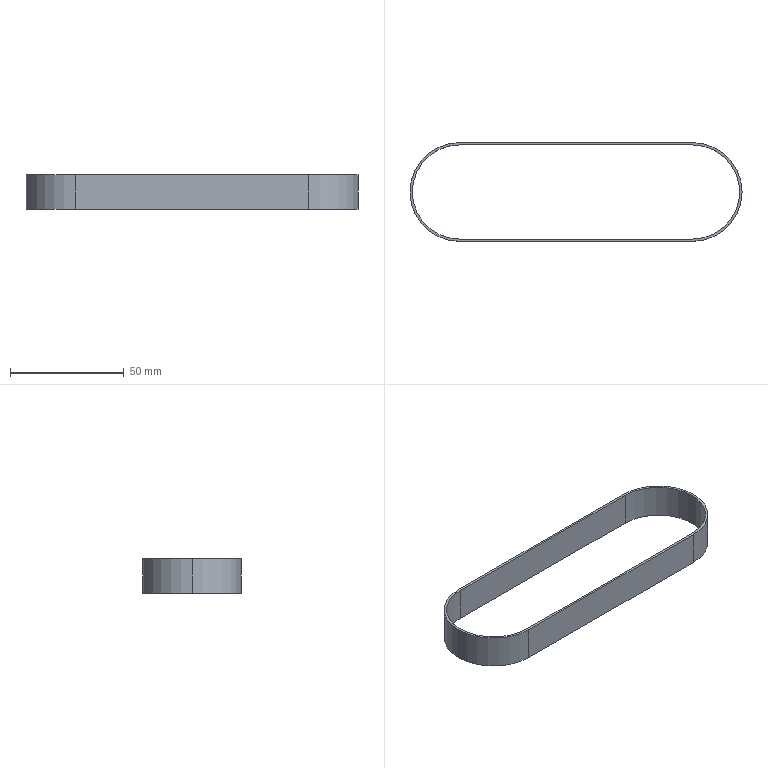Part | STEP file | Timing belt TTBU325T5-150_MISUMI | 1 solid | 12 faces | box 145.88 x 43.38 x 15 mm | volume 5072 mm3 | cylinder 6 | plane 6 | commonest cylinder face diameters 41.38 x3 43.38 x3
STEP:
#1=CARTESIAN_POINT('',(-21.69,0.,15.));
#2=VERTEX_POINT('',#1);
#3=CARTESIAN_POINT('',(0.,-21.69,15.));
#4=VERTEX_POINT('',#3);
#5=CARTESIAN_POINT('',(0.,0.,15.));
#6=DIRECTION('',(0.,0.,1.));
#7=DIRECTION('',(-1.,0.,0.));
#8=AXIS2_PLACEMENT_3D('',#5,#6,#7);
#9=CIRCLE('',#8,21.69);
#10=EDGE_CURVE('',#2,#4,#9,.T.);
#11=ORIENTED_EDGE('',*,*,#10,.F.);
#12=CARTESIAN_POINT('',(-21.69,0.,0.));
#13=VERTEX_POINT('',#12);
#14=CARTESIAN_POINT('',(-21.69,0.,15.));
#15=DIRECTION('',(0.,0.,-1.));
#16=VECTOR('',#15,1000.);
#17=LINE('',#14,#16);
#18=EDGE_CURVE('',#2,#13,#17,.T.);
#19=ORIENTED_EDGE('',*,*,#18,.T.);
#20=CARTESIAN_POINT('',(0.,-21.69,0.));
#21=VERTEX_POINT('',#20);
#22=CARTESIAN_POINT('',(0.,0.,0.));
#23=DIRECTION('',(0.,0.,1.));
#24=DIRECTION('',(-1.,0.,0.));
#25=AXIS2_PLACEMENT_3D('',#22,#23,#24);
#26=CIRCLE('',#25,21.69);
#27=EDGE_CURVE('',#13,#21,#26,.T.);
#28=ORIENTED_EDGE('',*,*,#27,.T.);
#29=CARTESIAN_POINT('',(0.,-21.69,15.));
#30=DIRECTION('',(0.,0.,1.));
#31=VECTOR('',#30,1000.);
#32=LINE('',#29,#31);
#33=EDGE_CURVE('',#21,#4,#32,.T.);
#34=ORIENTED_EDGE('',*,*,#33,.T.);
#35=EDGE_LOOP('',(#11,#19,#28,#34));
#36=FACE_OUTER_BOUND('',#35,.T.);
#37=CARTESIAN_POINT('',(0.,0.,15.));
#38=DIRECTION('',(0.,0.,-1.));
#39=DIRECTION('',(-1.,0.,0.));
#40=AXIS2_PLACEMENT_3D('',#37,#38,#39);
#41=CYLINDRICAL_SURFACE('',#40,21.69);
#42=ADVANCED_FACE('',(#36),#41,.T.);
#43=CARTESIAN_POINT('',(-20.69,0.,15.));
#44=VERTEX_POINT('',#43);
#45=CARTESIAN_POINT('',(0.,20.69,15.));
#46=VERTEX_POINT('',#45);
#47=CARTESIAN_POINT('',(0.,0.,15.));
#48=DIRECTION('',(0.,0.,-1.));
#49=DIRECTION('',(-1.,0.,0.));
#50=AXIS2_PLACEMENT_3D('',#47,#48,#49);
#51=CIRCLE('',#50,20.69);
#52=EDGE_CURVE('',#44,#46,#51,.T.);
#53=ORIENTED_EDGE('',*,*,#52,.F.);
#54=CARTESIAN_POINT('',(-20.69,0.,0.));
#55=VERTEX_POINT('',#54);
#56=CARTESIAN_POINT('',(-20.69,0.,15.));
#57=DIRECTION('',(0.,0.,-1.));
#58=VECTOR('',#57,1000.);
#59=LINE('',#56,#58);
#60=EDGE_CURVE('',#44,#55,#59,.T.);
#61=ORIENTED_EDGE('',*,*,#60,.T.);
#62=CARTESIAN_POINT('',(0.,20.69,0.));
#63=VERTEX_POINT('',#62);
#64=CARTESIAN_POINT('',(0.,0.,0.));
#65=DIRECTION('',(0.,0.,-1.));
#66=DIRECTION('',(-1.,0.,0.));
#67=AXIS2_PLACEMENT_3D('',#64,#65,#66);
#68=CIRCLE('',#67,20.69);
#69=EDGE_CURVE('',#55,#63,#68,.T.);
#70=ORIENTED_EDGE('',*,*,#69,.T.);
#71=CARTESIAN_POINT('',(0.,20.69,15.));
#72=DIRECTION('',(0.,0.,-1.));
#73=VECTOR('',#72,1000.);
#74=LINE('',#71,#73);
#75=EDGE_CURVE('',#46,#63,#74,.T.);
#76=ORIENTED_EDGE('',*,*,#75,.F.);
#77=EDGE_LOOP('',(#53,#61,#70,#76));
#78=FACE_OUTER_BOUND('',#77,.T.);
#79=CARTESIAN_POINT('',(0.,0.,15.));
#80=DIRECTION('',(0.,0.,-1.));
#81=DIRECTION('',(-1.,0.,0.));
#82=AXIS2_PLACEMENT_3D('',#79,#80,#81);
#83=CYLINDRICAL_SURFACE('',#82,20.69);
#84=ADVANCED_FACE('',(#78),#83,.F.);
#85=CARTESIAN_POINT('',(102.5,-21.69,15.));
#86=VERTEX_POINT('',#85);
#87=CARTESIAN_POINT('',(102.5,-21.69,0.));
#88=VERTEX_POINT('',#87);
#89=CARTESIAN_POINT('',(102.5,-21.69,15.));
#90=DIRECTION('',(0.,0.,-1.));
#91=VECTOR('',#90,1000.);
#92=LINE('',#89,#91);
#93=EDGE_CURVE('',#86,#88,#92,.T.);
#94=ORIENTED_EDGE('',*,*,#93,.F.);
#95=CARTESIAN_POINT('',(0.,-21.69,15.));
#96=DIRECTION('',(1.,0.,0.));
#97=VECTOR('',#96,1000.);
#98=LINE('',#95,#97);
#99=EDGE_CURVE('',#4,#86,#98,.T.);
#100=ORIENTED_EDGE('',*,*,#99,.F.);
#101=ORIENTED_EDGE('',*,*,#33,.F.);
#102=CARTESIAN_POINT('',(0.,-21.69,0.));
#103=DIRECTION('',(-1.,0.,0.));
#104=VECTOR('',#103,1000.);
#105=LINE('',#102,#104);
#106=EDGE_CURVE('',#88,#21,#105,.T.);
#107=ORIENTED_EDGE('',*,*,#106,.F.);
#108=EDGE_LOOP('',(#94,#100,#101,#107));
#109=FACE_OUTER_BOUND('',#108,.T.);
#110=CARTESIAN_POINT('',(0.,-21.69,15.));
#111=DIRECTION('',(0.,1.,0.));
#112=DIRECTION('',(0.,0.,1.));
#113=AXIS2_PLACEMENT_3D('',#110,#111,#112);
#114=PLANE('',#113);
#115=ADVANCED_FACE('',(#109),#114,.F.);
#116=CARTESIAN_POINT('',(0.,-20.69,0.));
#117=VERTEX_POINT('',#116);
#118=CARTESIAN_POINT('',(0.,0.,0.));
#119=DIRECTION('',(0.,0.,-1.));
#120=DIRECTION('',(-1.,0.,0.));
#121=AXIS2_PLACEMENT_3D('',#118,#119,#120);
#122=CIRCLE('',#121,20.69);
#123=EDGE_CURVE('',#117,#55,#122,.T.);
#124=ORIENTED_EDGE('',*,*,#123,.F.);
#125=CARTESIAN_POINT('',(102.5,-20.69,0.));
#126=VERTEX_POINT('',#125);
#127=CARTESIAN_POINT('',(0.,-20.69,0.));
#128=DIRECTION('',(-1.,0.,0.));
#129=VECTOR('',#128,1000.);
#130=LINE('',#127,#129);
#131=EDGE_CURVE('',#126,#117,#130,.T.);
#132=ORIENTED_EDGE('',*,*,#131,.F.);
#133=CARTESIAN_POINT('',(102.5,20.69,0.));
#134=VERTEX_POINT('',#133);
#135=CARTESIAN_POINT('',(102.5,0.,0.));
#136=DIRECTION('',(0.,0.,-1.));
#137=DIRECTION('',(-1.,0.,0.));
#138=AXIS2_PLACEMENT_3D('',#135,#136,#137);
#139=CIRCLE('',#138,20.69);
#140=EDGE_CURVE('',#134,#126,#139,.T.);
#141=ORIENTED_EDGE('',*,*,#140,.F.);
#142=CARTESIAN_POINT('',(0.,20.69,0.));
#143=DIRECTION('',(1.,0.,0.));
#144=VECTOR('',#143,1000.);
#145=LINE('',#142,#144);
#146=EDGE_CURVE('',#63,#134,#145,.T.);
#147=ORIENTED_EDGE('',*,*,#146,.F.);
#148=ORIENTED_EDGE('',*,*,#69,.F.);
#149=EDGE_LOOP('',(#124,#132,#141,#147,#148));
#150=FACE_BOUND('',#149,.T.);
#151=CARTESIAN_POINT('',(102.5,21.69,0.));
#152=VERTEX_POINT('',#151);
#153=CARTESIAN_POINT('',(0.,21.69,0.));
#154=VERTEX_POINT('',#153);
#155=CARTESIAN_POINT('',(0.,21.69,0.));
#156=DIRECTION('',(-1.,0.,0.));
#157=VECTOR('',#156,1000.);
#158=LINE('',#155,#157);
#159=EDGE_CURVE('',#152,#154,#158,.T.);
#160=ORIENTED_EDGE('',*,*,#159,.F.);
#161=CARTESIAN_POINT('',(102.5,0.,0.));
#162=DIRECTION('',(0.,0.,1.));
#163=DIRECTION('',(-1.,0.,0.));
#164=AXIS2_PLACEMENT_3D('',#161,#162,#163);
#165=CIRCLE('',#164,21.69);
#166=EDGE_CURVE('',#88,#152,#165,.T.);
#167=ORIENTED_EDGE('',*,*,#166,.F.);
#168=ORIENTED_EDGE('',*,*,#106,.T.);
#169=ORIENTED_EDGE('',*,*,#27,.F.);
#170=CARTESIAN_POINT('',(0.,0.,0.));
#171=DIRECTION('',(0.,0.,1.));
#172=DIRECTION('',(-1.,0.,0.));
#173=AXIS2_PLACEMENT_3D('',#170,#171,#172);
#174=CIRCLE('',#173,21.69);
#175=EDGE_CURVE('',#154,#13,#174,.T.);
#176=ORIENTED_EDGE('',*,*,#175,.F.);
#177=EDGE_LOOP('',(#160,#167,#168,#169,#176));
#178=FACE_OUTER_BOUND('',#177,.T.);
#179=CARTESIAN_POINT('',(0.,0.,0.));
#180=DIRECTION('',(0.,0.,1.));
#181=DIRECTION('',(1.,0.,0.));
#182=AXIS2_PLACEMENT_3D('',#179,#180,#181);
#183=PLANE('',#182);
#184=ADVANCED_FACE('',(#150,#178),#183,.F.);
#185=CARTESIAN_POINT('',(102.5,21.69,15.));
#186=VERTEX_POINT('',#185);
#187=CARTESIAN_POINT('',(102.5,0.,15.));
#188=DIRECTION('',(0.,0.,-1.));
#189=DIRECTION('',(-1.,0.,0.));
#190=AXIS2_PLACEMENT_3D('',#187,#188,#189);
#191=CIRCLE('',#190,21.69);
#192=EDGE_CURVE('',#186,#86,#191,.T.);
#193=ORIENTED_EDGE('',*,*,#192,.T.);
#194=ORIENTED_EDGE('',*,*,#93,.T.);
#195=ORIENTED_EDGE('',*,*,#166,.T.);
#196=CARTESIAN_POINT('',(102.5,21.69,15.));
#197=DIRECTION('',(0.,0.,1.));
#198=VECTOR('',#197,1000.);
#199=LINE('',#196,#198);
#200=EDGE_CURVE('',#152,#186,#199,.T.);
#201=ORIENTED_EDGE('',*,*,#200,.T.);
#202=EDGE_LOOP('',(#193,#194,#195,#201));
#203=FACE_OUTER_BOUND('',#202,.T.);
#204=CARTESIAN_POINT('',(102.5,0.,15.));
#205=DIRECTION('',(0.,0.,-1.));
#206=DIRECTION('',(-1.,0.,0.));
#207=AXIS2_PLACEMENT_3D('',#204,#205,#206);
#208=CYLINDRICAL_SURFACE('',#207,21.69);
#209=ADVANCED_FACE('',(#203),#208,.T.);
#210=CARTESIAN_POINT('',(102.5,20.69,15.));
#211=VERTEX_POINT('',#210);
#212=CARTESIAN_POINT('',(0.,20.69,15.));
#213=DIRECTION('',(1.,0.,0.));
#214=VECTOR('',#213,1000.);
#215=LINE('',#212,#214);
#216=EDGE_CURVE('',#46,#211,#215,.T.);
#217=ORIENTED_EDGE('',*,*,#216,.T.);
#218=CARTESIAN_POINT('',(102.5,-20.69,15.));
#219=VERTEX_POINT('',#218);
#220=CARTESIAN_POINT('',(102.5,0.,15.));
#221=DIRECTION('',(0.,0.,-1.));
#222=DIRECTION('',(-1.,0.,0.));
#223=AXIS2_PLACEMENT_3D('',#220,#221,#222);
#224=CIRCLE('',#223,20.69);
#225=EDGE_CURVE('',#211,#219,#224,.T.);
#226=ORIENTED_EDGE('',*,*,#225,.T.);
#227=CARTESIAN_POINT('',(0.,-20.69,15.));
#228=VERTEX_POINT('',#227);
#229=CARTESIAN_POINT('',(0.,-20.69,15.));
#230=DIRECTION('',(-1.,0.,0.));
#231=VECTOR('',#230,1000.);
#232=LINE('',#229,#231);
#233=EDGE_CURVE('',#219,#228,#232,.T.);
#234=ORIENTED_EDGE('',*,*,#233,.T.);
#235=CARTESIAN_POINT('',(0.,0.,15.));
#236=DIRECTION('',(0.,0.,-1.));
#237=DIRECTION('',(-1.,0.,0.));
#238=AXIS2_PLACEMENT_3D('',#235,#236,#237);
#239=CIRCLE('',#238,20.69);
#240=EDGE_CURVE('',#228,#44,#239,.T.);
#241=ORIENTED_EDGE('',*,*,#240,.T.);
#242=ORIENTED_EDGE('',*,*,#52,.T.);
#243=EDGE_LOOP('',(#217,#226,#234,#241,#242));
#244=FACE_BOUND('',#243,.T.);
#245=ORIENTED_EDGE('',*,*,#192,.F.);
#246=CARTESIAN_POINT('',(0.,21.69,15.));
#247=VERTEX_POINT('',#246);
#248=CARTESIAN_POINT('',(0.,21.69,15.));
#249=DIRECTION('',(-1.,0.,0.));
#250=VECTOR('',#249,1000.);
#251=LINE('',#248,#250);
#252=EDGE_CURVE('',#186,#247,#251,.T.);
#253=ORIENTED_EDGE('',*,*,#252,.T.);
#254=CARTESIAN_POINT('',(0.,0.,15.));
#255=DIRECTION('',(0.,0.,1.));
#256=DIRECTION('',(-1.,0.,0.));
#257=AXIS2_PLACEMENT_3D('',#254,#255,#256);
#258=CIRCLE('',#257,21.69);
#259=EDGE_CURVE('',#247,#2,#258,.T.);
#260=ORIENTED_EDGE('',*,*,#259,.T.);
#261=ORIENTED_EDGE('',*,*,#10,.T.);
#262=ORIENTED_EDGE('',*,*,#99,.T.);
#263=EDGE_LOOP('',(#245,#253,#260,#261,#262));
#264=FACE_OUTER_BOUND('',#263,.T.);
#265=CARTESIAN_POINT('',(0.,0.,15.));
#266=DIRECTION('',(0.,0.,1.));
#267=DIRECTION('',(1.,0.,0.));
#268=AXIS2_PLACEMENT_3D('',#265,#266,#267);
#269=PLANE('',#268);
#270=ADVANCED_FACE('',(#244,#264),#269,.T.);
#271=ORIENTED_EDGE('',*,*,#18,.F.);
#272=ORIENTED_EDGE('',*,*,#259,.F.);
#273=CARTESIAN_POINT('',(0.,21.69,15.));
#274=DIRECTION('',(0.,0.,-1.));
#275=VECTOR('',#274,1000.);
#276=LINE('',#273,#275);
#277=EDGE_CURVE('',#247,#154,#276,.T.);
#278=ORIENTED_EDGE('',*,*,#277,.T.);
#279=ORIENTED_EDGE('',*,*,#175,.T.);
#280=EDGE_LOOP('',(#271,#272,#278,#279));
#281=FACE_OUTER_BOUND('',#280,.T.);
#282=CARTESIAN_POINT('',(0.,0.,15.));
#283=DIRECTION('',(0.,0.,-1.));
#284=DIRECTION('',(-1.,0.,0.));
#285=AXIS2_PLACEMENT_3D('',#282,#283,#284);
#286=CYLINDRICAL_SURFACE('',#285,21.69);
#287=ADVANCED_FACE('',(#281),#286,.T.);
#288=ORIENTED_EDGE('',*,*,#60,.F.);
#289=ORIENTED_EDGE('',*,*,#240,.F.);
#290=CARTESIAN_POINT('',(0.,-20.69,15.));
#291=DIRECTION('',(0.,0.,1.));
#292=VECTOR('',#291,1000.);
#293=LINE('',#290,#292);
#294=EDGE_CURVE('',#117,#228,#293,.T.);
#295=ORIENTED_EDGE('',*,*,#294,.F.);
#296=ORIENTED_EDGE('',*,*,#123,.T.);
#297=EDGE_LOOP('',(#288,#289,#295,#296));
#298=FACE_OUTER_BOUND('',#297,.T.);
#299=CARTESIAN_POINT('',(0.,0.,15.));
#300=DIRECTION('',(0.,0.,-1.));
#301=DIRECTION('',(-1.,0.,0.));
#302=AXIS2_PLACEMENT_3D('',#299,#300,#301);
#303=CYLINDRICAL_SURFACE('',#302,20.69);
#304=ADVANCED_FACE('',(#298),#303,.F.);
#305=ORIENTED_EDGE('',*,*,#233,.F.);
#306=CARTESIAN_POINT('',(102.5,-20.69,15.));
#307=DIRECTION('',(0.,0.,-1.));
#308=VECTOR('',#307,1000.);
#309=LINE('',#306,#308);
#310=EDGE_CURVE('',#219,#126,#309,.T.);
#311=ORIENTED_EDGE('',*,*,#310,.T.);
#312=ORIENTED_EDGE('',*,*,#131,.T.);
#313=ORIENTED_EDGE('',*,*,#294,.T.);
#314=EDGE_LOOP('',(#305,#311,#312,#313));
#315=FACE_OUTER_BOUND('',#314,.T.);
#316=CARTESIAN_POINT('',(0.,-20.69,15.));
#317=DIRECTION('',(0.,1.,0.));
#318=DIRECTION('',(0.,0.,1.));
#319=AXIS2_PLACEMENT_3D('',#316,#317,#318);
#320=PLANE('',#319);
#321=ADVANCED_FACE('',(#315),#320,.T.);
#322=ORIENTED_EDGE('',*,*,#310,.F.);
#323=ORIENTED_EDGE('',*,*,#225,.F.);
#324=CARTESIAN_POINT('',(102.5,20.69,15.));
#325=DIRECTION('',(0.,0.,1.));
#326=VECTOR('',#325,1000.);
#327=LINE('',#324,#326);
#328=EDGE_CURVE('',#134,#211,#327,.T.);
#329=ORIENTED_EDGE('',*,*,#328,.F.);
#330=ORIENTED_EDGE('',*,*,#140,.T.);
#331=EDGE_LOOP('',(#322,#323,#329,#330));
#332=FACE_OUTER_BOUND('',#331,.T.);
#333=CARTESIAN_POINT('',(102.5,0.,15.));
#334=DIRECTION('',(0.,0.,-1.));
#335=DIRECTION('',(-1.,0.,0.));
#336=AXIS2_PLACEMENT_3D('',#333,#334,#335);
#337=CYLINDRICAL_SURFACE('',#336,20.69);
#338=ADVANCED_FACE('',(#332),#337,.F.);
#339=ORIENTED_EDGE('',*,*,#216,.F.);
#340=ORIENTED_EDGE('',*,*,#75,.T.);
#341=ORIENTED_EDGE('',*,*,#146,.T.);
#342=ORIENTED_EDGE('',*,*,#328,.T.);
#343=EDGE_LOOP('',(#339,#340,#341,#342));
#344=FACE_OUTER_BOUND('',#343,.T.);
#345=CARTESIAN_POINT('',(0.,20.69,15.));
#346=DIRECTION('',(0.,-1.,0.));
#347=DIRECTION('',(0.,0.,-1.));
#348=AXIS2_PLACEMENT_3D('',#345,#346,#347);
#349=PLANE('',#348);
#350=ADVANCED_FACE('',(#344),#349,.T.);
#351=ORIENTED_EDGE('',*,*,#277,.F.);
#352=ORIENTED_EDGE('',*,*,#252,.F.);
#353=ORIENTED_EDGE('',*,*,#200,.F.);
#354=ORIENTED_EDGE('',*,*,#159,.T.);
#355=EDGE_LOOP('',(#351,#352,#353,#354));
#356=FACE_OUTER_BOUND('',#355,.T.);
#357=CARTESIAN_POINT('',(0.,21.69,15.));
#358=DIRECTION('',(0.,-1.,0.));
#359=DIRECTION('',(0.,0.,-1.));
#360=AXIS2_PLACEMENT_3D('',#357,#358,#359);
#361=PLANE('',#360);
#362=ADVANCED_FACE('',(#356),#361,.F.);
#363=CLOSED_SHELL('',(#42,#84,#115,#184,#209,#270,#287,#304,#321,#338,#350,#362));
#364=MANIFOLD_SOLID_BREP('',#363);
#365=CARTESIAN_POINT('',(0.,0.,0.));
#366=DIRECTION('',(0.,0.,1.));
#367=DIRECTION('',(1.,0.,0.));
#368=AXIS2_PLACEMENT_3D('',#365,#366,#367);
#369=(LENGTH_UNIT()NAMED_UNIT(*)SI_UNIT(.MILLI.,.METRE.));
#370=UNCERTAINTY_MEASURE_WITH_UNIT(LENGTH_MEASURE(0.00001),#369,'','');
#371=(NAMED_UNIT(*)PLANE_ANGLE_UNIT()SI_UNIT($,.RADIAN.));
#372=(NAMED_UNIT(*)SI_UNIT($,.STERADIAN.)SOLID_ANGLE_UNIT());
#373=(GEOMETRIC_REPRESENTATION_CONTEXT(3)GLOBAL_UNCERTAINTY_ASSIGNED_CONTEXT((#370))GLOBAL_UNIT_ASSIGNED_CONTEXT((#369,#371,#372))REPRESENTATION_CONTEXT('',''));
#374=ADVANCED_BREP_SHAPE_REPRESENTATION('',(#364,#368),#373);